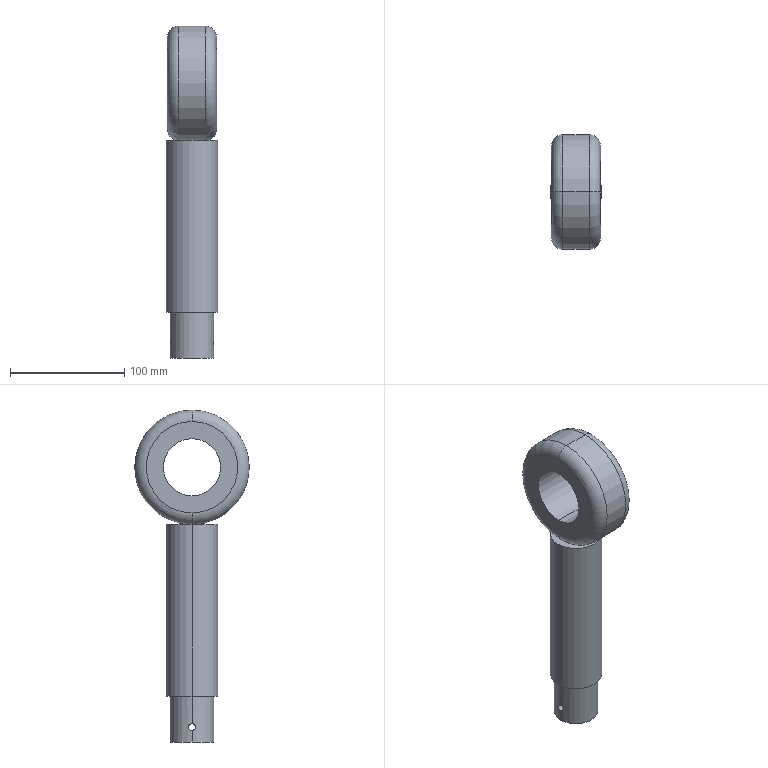Part | SolidWorks | features ICE 3, Extrusion 1, Fillet 1 | 2 solids | 19 faces | box 45 x 100 x 290 mm | volume 523268 mm3 | cylinder 10 | plane 5 | torus 4 | commonest cylinder face diameters 6 x2 38 x2 45 x2 50 x2 100 x2
STEP:
#1=CARTESIAN_POINT('',(11.5,0.,290.));
#2=VERTEX_POINT('',#1);
#3=CARTESIAN_POINT('',(11.5,0.,190.));
#4=VERTEX_POINT('',#3);
#5=CARTESIAN_POINT('',(11.5,0.,240.));
#6=DIRECTION('',(-1.,0.,0.));
#7=DIRECTION('',(0.,0.,-1.));
#8=AXIS2_PLACEMENT_3D('',#5,#6,#7);
#9=CIRCLE('',#8,50.);
#10=EDGE_CURVE('',#2,#4,#9,.T.);
#11=ORIENTED_EDGE('',*,*,#10,.F.);
#12=CARTESIAN_POINT('',(21.5,0.,280.));
#13=VERTEX_POINT('',#12);
#14=CARTESIAN_POINT('',(11.5,0.,280.));
#15=DIRECTION('',(0.,1.,0.));
#16=DIRECTION('',(0.,0.,1.));
#17=AXIS2_PLACEMENT_3D('',#14,#15,#16);
#18=CIRCLE('',#17,10.);
#19=EDGE_CURVE('',#2,#13,#18,.T.);
#20=ORIENTED_EDGE('',*,*,#19,.T.);
#21=CARTESIAN_POINT('',(21.5,0.,200.));
#22=VERTEX_POINT('',#21);
#23=CARTESIAN_POINT('',(21.5,0.,240.));
#24=DIRECTION('',(1.,0.,0.));
#25=DIRECTION('',(0.,0.,-1.));
#26=AXIS2_PLACEMENT_3D('',#23,#24,#25);
#27=CIRCLE('',#26,40.);
#28=EDGE_CURVE('',#22,#13,#27,.T.);
#29=ORIENTED_EDGE('',*,*,#28,.F.);
#30=CARTESIAN_POINT('',(11.5,0.,200.));
#31=DIRECTION('',(0.,-1.,0.));
#32=DIRECTION('',(0.,0.,-1.));
#33=AXIS2_PLACEMENT_3D('',#30,#31,#32);
#34=CIRCLE('',#33,10.);
#35=EDGE_CURVE('',#4,#22,#34,.T.);
#36=ORIENTED_EDGE('',*,*,#35,.F.);
#37=EDGE_LOOP('',(#11,#20,#29,#36));
#38=FACE_OUTER_BOUND('',#37,.T.);
#39=CARTESIAN_POINT('',(11.5,0.,240.));
#40=DIRECTION('',(1.,0.,0.));
#41=DIRECTION('',(0.,0.,-1.));
#42=AXIS2_PLACEMENT_3D('',#39,#40,#41);
#43=TOROIDAL_SURFACE('',#42,40.,10.);
#44=ADVANCED_FACE('',(#38),#43,.T.);
#45=CARTESIAN_POINT('',(-21.5,0.,280.));
#46=VERTEX_POINT('',#45);
#47=CARTESIAN_POINT('',(-21.5,0.,200.));
#48=VERTEX_POINT('',#47);
#49=CARTESIAN_POINT('',(-21.5,0.,240.));
#50=DIRECTION('',(-1.,0.,0.));
#51=DIRECTION('',(0.,0.,-1.));
#52=AXIS2_PLACEMENT_3D('',#49,#50,#51);
#53=CIRCLE('',#52,40.);
#54=EDGE_CURVE('',#46,#48,#53,.T.);
#55=ORIENTED_EDGE('',*,*,#54,.F.);
#56=CARTESIAN_POINT('',(-11.5,0.,290.));
#57=VERTEX_POINT('',#56);
#58=CARTESIAN_POINT('',(-11.5,0.,280.));
#59=DIRECTION('',(0.,1.,0.));
#60=DIRECTION('',(0.,0.,1.));
#61=AXIS2_PLACEMENT_3D('',#58,#59,#60);
#62=CIRCLE('',#61,10.);
#63=EDGE_CURVE('',#46,#57,#62,.T.);
#64=ORIENTED_EDGE('',*,*,#63,.T.);
#65=CARTESIAN_POINT('',(-11.5,0.,190.));
#66=VERTEX_POINT('',#65);
#67=CARTESIAN_POINT('',(-11.5,0.,240.));
#68=DIRECTION('',(1.,0.,0.));
#69=DIRECTION('',(0.,0.,-1.));
#70=AXIS2_PLACEMENT_3D('',#67,#68,#69);
#71=CIRCLE('',#70,50.);
#72=EDGE_CURVE('',#66,#57,#71,.T.);
#73=ORIENTED_EDGE('',*,*,#72,.F.);
#74=CARTESIAN_POINT('',(-11.5,0.,200.));
#75=DIRECTION('',(0.,-1.,0.));
#76=DIRECTION('',(0.,0.,-1.));
#77=AXIS2_PLACEMENT_3D('',#74,#75,#76);
#78=CIRCLE('',#77,10.);
#79=EDGE_CURVE('',#48,#66,#78,.T.);
#80=ORIENTED_EDGE('',*,*,#79,.F.);
#81=EDGE_LOOP('',(#55,#64,#73,#80));
#82=FACE_OUTER_BOUND('',#81,.T.);
#83=CARTESIAN_POINT('',(-11.5,0.,240.));
#84=DIRECTION('',(1.,0.,0.));
#85=DIRECTION('',(0.,0.,-1.));
#86=AXIS2_PLACEMENT_3D('',#83,#84,#85);
#87=TOROIDAL_SURFACE('',#86,40.,10.);
#88=ADVANCED_FACE('',(#82),#87,.T.);
#89=CARTESIAN_POINT('',(21.5,0.,265.));
#90=VERTEX_POINT('',#89);
#91=CARTESIAN_POINT('',(21.5,0.,215.));
#92=VERTEX_POINT('',#91);
#93=CARTESIAN_POINT('',(21.5,0.,240.));
#94=DIRECTION('',(1.,0.,0.));
#95=DIRECTION('',(0.,0.,-1.));
#96=AXIS2_PLACEMENT_3D('',#93,#94,#95);
#97=CIRCLE('',#96,25.);
#98=EDGE_CURVE('',#90,#92,#97,.T.);
#99=ORIENTED_EDGE('',*,*,#98,.T.);
#100=CARTESIAN_POINT('',(-21.5,0.,215.));
#101=VERTEX_POINT('',#100);
#102=CARTESIAN_POINT('',(21.5,0.,215.));
#103=DIRECTION('',(-1.,0.,0.));
#104=VECTOR('',#103,1000.);
#105=LINE('',#102,#104);
#106=EDGE_CURVE('',#92,#101,#105,.T.);
#107=ORIENTED_EDGE('',*,*,#106,.T.);
#108=CARTESIAN_POINT('',(-21.5,0.,265.));
#109=VERTEX_POINT('',#108);
#110=CARTESIAN_POINT('',(-21.5,0.,240.));
#111=DIRECTION('',(1.,0.,0.));
#112=DIRECTION('',(0.,0.,-1.));
#113=AXIS2_PLACEMENT_3D('',#110,#111,#112);
#114=CIRCLE('',#113,25.);
#115=EDGE_CURVE('',#109,#101,#114,.T.);
#116=ORIENTED_EDGE('',*,*,#115,.F.);
#117=CARTESIAN_POINT('',(21.5,0.,265.));
#118=DIRECTION('',(-1.,0.,0.));
#119=VECTOR('',#118,1000.);
#120=LINE('',#117,#119);
#121=EDGE_CURVE('',#90,#109,#120,.T.);
#122=ORIENTED_EDGE('',*,*,#121,.F.);
#123=EDGE_LOOP('',(#99,#107,#116,#122));
#124=FACE_OUTER_BOUND('',#123,.T.);
#125=CARTESIAN_POINT('',(21.5,0.,240.));
#126=DIRECTION('',(-1.,0.,0.));
#127=DIRECTION('',(0.,0.,1.));
#128=AXIS2_PLACEMENT_3D('',#125,#126,#127);
#129=CYLINDRICAL_SURFACE('',#128,25.);
#130=ADVANCED_FACE('',(#124),#129,.F.);
#131=ORIENTED_EDGE('',*,*,#10,.T.);
#132=CARTESIAN_POINT('',(21.5,0.,190.));
#133=DIRECTION('',(-1.,0.,0.));
#134=VECTOR('',#133,1000.);
#135=LINE('',#132,#134);
#136=EDGE_CURVE('',#4,#66,#135,.T.);
#137=ORIENTED_EDGE('',*,*,#136,.T.);
#138=ORIENTED_EDGE('',*,*,#72,.T.);
#139=CARTESIAN_POINT('',(21.5,0.,290.));
#140=DIRECTION('',(-1.,0.,0.));
#141=VECTOR('',#140,1000.);
#142=LINE('',#139,#141);
#143=EDGE_CURVE('',#2,#57,#142,.T.);
#144=ORIENTED_EDGE('',*,*,#143,.F.);
#145=EDGE_LOOP('',(#131,#137,#138,#144));
#146=FACE_OUTER_BOUND('',#145,.T.);
#147=CARTESIAN_POINT('',(21.5,0.,240.));
#148=DIRECTION('',(-1.,0.,0.));
#149=DIRECTION('',(0.,0.,1.));
#150=AXIS2_PLACEMENT_3D('',#147,#148,#149);
#151=CYLINDRICAL_SURFACE('',#150,50.);
#152=ADVANCED_FACE('',(#146),#151,.T.);
#153=ORIENTED_EDGE('',*,*,#28,.T.);
#154=CARTESIAN_POINT('',(21.5,0.,240.));
#155=DIRECTION('',(1.,0.,0.));
#156=DIRECTION('',(0.,0.,-1.));
#157=AXIS2_PLACEMENT_3D('',#154,#155,#156);
#158=CIRCLE('',#157,40.);
#159=EDGE_CURVE('',#13,#22,#158,.T.);
#160=ORIENTED_EDGE('',*,*,#159,.T.);
#161=EDGE_LOOP('',(#153,#160));
#162=FACE_OUTER_BOUND('',#161,.T.);
#163=ORIENTED_EDGE('',*,*,#98,.F.);
#164=CARTESIAN_POINT('',(21.5,0.,240.));
#165=DIRECTION('',(1.,0.,0.));
#166=DIRECTION('',(0.,0.,-1.));
#167=AXIS2_PLACEMENT_3D('',#164,#165,#166);
#168=CIRCLE('',#167,25.);
#169=EDGE_CURVE('',#92,#90,#168,.T.);
#170=ORIENTED_EDGE('',*,*,#169,.F.);
#171=EDGE_LOOP('',(#163,#170));
#172=FACE_BOUND('',#171,.T.);
#173=CARTESIAN_POINT('',(21.5,0.,240.));
#174=DIRECTION('',(1.,0.,0.));
#175=DIRECTION('',(0.,0.,-1.));
#176=AXIS2_PLACEMENT_3D('',#173,#174,#175);
#177=PLANE('',#176);
#178=ADVANCED_FACE('',(#162,#172),#177,.T.);
#179=CARTESIAN_POINT('',(-21.5,0.,240.));
#180=DIRECTION('',(-1.,0.,0.));
#181=DIRECTION('',(0.,0.,-1.));
#182=AXIS2_PLACEMENT_3D('',#179,#180,#181);
#183=CIRCLE('',#182,40.);
#184=EDGE_CURVE('',#48,#46,#183,.T.);
#185=ORIENTED_EDGE('',*,*,#184,.T.);
#186=ORIENTED_EDGE('',*,*,#54,.T.);
#187=EDGE_LOOP('',(#185,#186));
#188=FACE_OUTER_BOUND('',#187,.T.);
#189=ORIENTED_EDGE('',*,*,#115,.T.);
#190=CARTESIAN_POINT('',(-21.5,0.,240.));
#191=DIRECTION('',(1.,0.,0.));
#192=DIRECTION('',(0.,0.,-1.));
#193=AXIS2_PLACEMENT_3D('',#190,#191,#192);
#194=CIRCLE('',#193,25.);
#195=EDGE_CURVE('',#101,#109,#194,.T.);
#196=ORIENTED_EDGE('',*,*,#195,.T.);
#197=EDGE_LOOP('',(#189,#196));
#198=FACE_BOUND('',#197,.T.);
#199=CARTESIAN_POINT('',(-21.5,0.,240.));
#200=DIRECTION('',(1.,0.,0.));
#201=DIRECTION('',(0.,0.,-1.));
#202=AXIS2_PLACEMENT_3D('',#199,#200,#201);
#203=PLANE('',#202);
#204=ADVANCED_FACE('',(#188,#198),#203,.F.);
#205=ORIENTED_EDGE('',*,*,#136,.F.);
#206=CARTESIAN_POINT('',(11.5,0.,240.));
#207=DIRECTION('',(-1.,0.,0.));
#208=DIRECTION('',(0.,0.,-1.));
#209=AXIS2_PLACEMENT_3D('',#206,#207,#208);
#210=CIRCLE('',#209,50.);
#211=EDGE_CURVE('',#4,#2,#210,.T.);
#212=ORIENTED_EDGE('',*,*,#211,.T.);
#213=ORIENTED_EDGE('',*,*,#143,.T.);
#214=CARTESIAN_POINT('',(-11.5,0.,240.));
#215=DIRECTION('',(1.,0.,0.));
#216=DIRECTION('',(0.,0.,-1.));
#217=AXIS2_PLACEMENT_3D('',#214,#215,#216);
#218=CIRCLE('',#217,50.);
#219=EDGE_CURVE('',#57,#66,#218,.T.);
#220=ORIENTED_EDGE('',*,*,#219,.T.);
#221=EDGE_LOOP('',(#205,#212,#213,#220));
#222=FACE_OUTER_BOUND('',#221,.T.);
#223=CARTESIAN_POINT('',(21.5,0.,240.));
#224=DIRECTION('',(-1.,0.,0.));
#225=DIRECTION('',(0.,0.,1.));
#226=AXIS2_PLACEMENT_3D('',#223,#224,#225);
#227=CYLINDRICAL_SURFACE('',#226,50.);
#228=ADVANCED_FACE('',(#222),#227,.T.);
#229=ORIENTED_EDGE('',*,*,#106,.F.);
#230=ORIENTED_EDGE('',*,*,#169,.T.);
#231=ORIENTED_EDGE('',*,*,#121,.T.);
#232=ORIENTED_EDGE('',*,*,#195,.F.);
#233=EDGE_LOOP('',(#229,#230,#231,#232));
#234=FACE_OUTER_BOUND('',#233,.T.);
#235=CARTESIAN_POINT('',(21.5,0.,240.));
#236=DIRECTION('',(-1.,0.,0.));
#237=DIRECTION('',(0.,0.,1.));
#238=AXIS2_PLACEMENT_3D('',#235,#236,#237);
#239=CYLINDRICAL_SURFACE('',#238,25.);
#240=ADVANCED_FACE('',(#234),#239,.F.);
#241=ORIENTED_EDGE('',*,*,#63,.F.);
#242=ORIENTED_EDGE('',*,*,#184,.F.);
#243=ORIENTED_EDGE('',*,*,#79,.T.);
#244=ORIENTED_EDGE('',*,*,#219,.F.);
#245=EDGE_LOOP('',(#241,#242,#243,#244));
#246=FACE_OUTER_BOUND('',#245,.T.);
#247=CARTESIAN_POINT('',(-11.5,0.,240.));
#248=DIRECTION('',(1.,0.,0.));
#249=DIRECTION('',(0.,0.,-1.));
#250=AXIS2_PLACEMENT_3D('',#247,#248,#249);
#251=TOROIDAL_SURFACE('',#250,40.,10.);
#252=ADVANCED_FACE('',(#246),#251,.T.);
#253=ORIENTED_EDGE('',*,*,#19,.F.);
#254=ORIENTED_EDGE('',*,*,#211,.F.);
#255=ORIENTED_EDGE('',*,*,#35,.T.);
#256=ORIENTED_EDGE('',*,*,#159,.F.);
#257=EDGE_LOOP('',(#253,#254,#255,#256));
#258=FACE_OUTER_BOUND('',#257,.T.);
#259=CARTESIAN_POINT('',(11.5,0.,240.));
#260=DIRECTION('',(1.,0.,0.));
#261=DIRECTION('',(0.,0.,-1.));
#262=AXIS2_PLACEMENT_3D('',#259,#260,#261);
#263=TOROIDAL_SURFACE('',#262,40.,10.);
#264=ADVANCED_FACE('',(#258),#263,.T.);
#265=CLOSED_SHELL('',(#44,#88,#130,#152,#178,#204,#228,#240,#252,#264));
#266=MANIFOLD_SOLID_BREP('',#265);
#267=CARTESIAN_POINT('',(-19.,0.,10.));
#268=VERTEX_POINT('',#267);
#269=CARTESIAN_POINT('',(-19.,0.,16.));
#270=VERTEX_POINT('',#269);
#271=CARTESIAN_POINT('',(-19.,0.,10.));
#272=CARTESIAN_POINT('',(-19.,-0.1959,10.));
#273=CARTESIAN_POINT('',(-18.997,-0.3908,10.019));
#274=CARTESIAN_POINT('',(-18.985,-0.7787,10.096));
#275=CARTESIAN_POINT('',(-18.976,-0.9676,10.154));
#276=CARTESIAN_POINT('',(-18.954,-1.329,10.303));
#277=CARTESIAN_POINT('',(-18.941,-1.504,10.397));
#278=CARTESIAN_POINT('',(-18.912,-1.831,10.615));
#279=CARTESIAN_POINT('',(-18.897,-1.982,10.739));
#280=CARTESIAN_POINT('',(-18.866,-2.258,11.015));
#281=CARTESIAN_POINT('',(-18.85,-2.385,11.17));
#282=CARTESIAN_POINT('',(-18.821,-2.602,11.495));
#283=CARTESIAN_POINT('',(-18.808,-2.695,11.667));
#284=CARTESIAN_POINT('',(-18.786,-2.846,12.03));
#285=CARTESIAN_POINT('',(-18.777,-2.904,12.221));
#286=CARTESIAN_POINT('',(-18.765,-2.98,12.604));
#287=CARTESIAN_POINT('',(-18.762,-3.,12.8));
#288=CARTESIAN_POINT('',(-18.762,-3.,13.196));
#289=CARTESIAN_POINT('',(-18.765,-2.981,13.391));
#290=CARTESIAN_POINT('',(-18.777,-2.905,13.775));
#291=CARTESIAN_POINT('',(-18.786,-2.847,13.966));
#292=CARTESIAN_POINT('',(-18.808,-2.697,14.329));
#293=CARTESIAN_POINT('',(-18.821,-2.605,14.501));
#294=CARTESIAN_POINT('',(-18.85,-2.387,14.828));
#295=CARTESIAN_POINT('',(-18.866,-2.261,14.982));
#296=CARTESIAN_POINT('',(-18.897,-1.985,15.258));
#297=CARTESIAN_POINT('',(-18.912,-1.834,15.382));
#298=CARTESIAN_POINT('',(-18.941,-1.506,15.602));
#299=CARTESIAN_POINT('',(-18.954,-1.332,15.695));
#300=CARTESIAN_POINT('',(-18.976,-0.9717,15.845));
#301=CARTESIAN_POINT('',(-18.985,-0.7822,15.903));
#302=CARTESIAN_POINT('',(-18.997,-0.3946,15.98));
#303=CARTESIAN_POINT('',(-19.,-0.1985,16.));
#304=CARTESIAN_POINT('',(-19.,0.,16.));
#305=B_SPLINE_CURVE_WITH_KNOTS('',3,(#271,#272,#273,#274,#275,#276,#277,#278,#279,#280,#281,#282,#283,#284,#285,#286,#287,#288,#289,#290,#291,#292,#293,#294,#295,#296,#297,#298,#299,#300,#301,#302,#303,#304),.UNSPECIFIED.,.F.,.F.,(4,2,2,2,2,2,2,2,2,2,2,2,2,2,2,2,4),(0.009394,0.009981,0.01057,0.01116,0.01174,0.01233,0.01292,0.0135,0.01409,0.01468,0.01526,0.01585,0.01644,0.01702,0.01761,0.0182,0.01879),.UNSPECIFIED.);
#306=EDGE_CURVE('',#268,#270,#305,.T.);
#307=ORIENTED_EDGE('',*,*,#306,.T.);
#308=CARTESIAN_POINT('',(19.,0.,16.));
#309=VERTEX_POINT('',#308);
#310=CARTESIAN_POINT('',(-25.,0.,16.));
#311=DIRECTION('',(1.,0.,0.));
#312=VECTOR('',#311,1000.);
#313=LINE('',#310,#312);
#314=EDGE_CURVE('',#270,#309,#313,.T.);
#315=ORIENTED_EDGE('',*,*,#314,.T.);
#316=CARTESIAN_POINT('',(19.,0.,10.));
#317=VERTEX_POINT('',#316);
#318=CARTESIAN_POINT('',(19.,0.,16.));
#319=CARTESIAN_POINT('',(19.,-0.1959,16.));
#320=CARTESIAN_POINT('',(18.997,-0.3908,15.981));
#321=CARTESIAN_POINT('',(18.985,-0.7787,15.904));
#322=CARTESIAN_POINT('',(18.976,-0.9676,15.846));
#323=CARTESIAN_POINT('',(18.954,-1.329,15.697));
#324=CARTESIAN_POINT('',(18.941,-1.504,15.603));
#325=CARTESIAN_POINT('',(18.912,-1.831,15.385));
#326=CARTESIAN_POINT('',(18.897,-1.982,15.261));
#327=CARTESIAN_POINT('',(18.866,-2.258,14.985));
#328=CARTESIAN_POINT('',(18.85,-2.385,14.83));
#329=CARTESIAN_POINT('',(18.821,-2.602,14.505));
#330=CARTESIAN_POINT('',(18.808,-2.695,14.333));
#331=CARTESIAN_POINT('',(18.786,-2.846,13.97));
#332=CARTESIAN_POINT('',(18.777,-2.904,13.779));
#333=CARTESIAN_POINT('',(18.765,-2.98,13.396));
#334=CARTESIAN_POINT('',(18.762,-3.,13.2));
#335=CARTESIAN_POINT('',(18.762,-3.,12.804));
#336=CARTESIAN_POINT('',(18.765,-2.981,12.609));
#337=CARTESIAN_POINT('',(18.777,-2.905,12.225));
#338=CARTESIAN_POINT('',(18.786,-2.847,12.034));
#339=CARTESIAN_POINT('',(18.808,-2.697,11.671));
#340=CARTESIAN_POINT('',(18.821,-2.605,11.499));
#341=CARTESIAN_POINT('',(18.85,-2.387,11.172));
#342=CARTESIAN_POINT('',(18.866,-2.261,11.018));
#343=CARTESIAN_POINT('',(18.897,-1.985,10.742));
#344=CARTESIAN_POINT('',(18.912,-1.834,10.618));
#345=CARTESIAN_POINT('',(18.941,-1.506,10.398));
#346=CARTESIAN_POINT('',(18.954,-1.332,10.305));
#347=CARTESIAN_POINT('',(18.976,-0.9717,10.155));
#348=CARTESIAN_POINT('',(18.985,-0.7822,10.097));
#349=CARTESIAN_POINT('',(18.997,-0.3946,10.02));
#350=CARTESIAN_POINT('',(19.,-0.1985,10.));
#351=CARTESIAN_POINT('',(19.,0.,10.));
#352=B_SPLINE_CURVE_WITH_KNOTS('',3,(#318,#319,#320,#321,#322,#323,#324,#325,#326,#327,#328,#329,#330,#331,#332,#333,#334,#335,#336,#337,#338,#339,#340,#341,#342,#343,#344,#345,#346,#347,#348,#349,#350,#351),.UNSPECIFIED.,.F.,.F.,(4,2,2,2,2,2,2,2,2,2,2,2,2,2,2,2,4),(0.009394,0.009981,0.01057,0.01116,0.01174,0.01233,0.01292,0.0135,0.01409,0.01468,0.01526,0.01585,0.01644,0.01702,0.01761,0.0182,0.01879),.UNSPECIFIED.);
#353=EDGE_CURVE('',#309,#317,#352,.T.);
#354=ORIENTED_EDGE('',*,*,#353,.T.);
#355=CARTESIAN_POINT('',(-25.,0.,10.));
#356=DIRECTION('',(1.,0.,0.));
#357=VECTOR('',#356,1000.);
#358=LINE('',#355,#357);
#359=EDGE_CURVE('',#268,#317,#358,.T.);
#360=ORIENTED_EDGE('',*,*,#359,.F.);
#361=EDGE_LOOP('',(#307,#315,#354,#360));
#362=FACE_OUTER_BOUND('',#361,.T.);
#363=CARTESIAN_POINT('',(-25.,0.,13.));
#364=DIRECTION('',(1.,0.,0.));
#365=DIRECTION('',(0.,0.,-1.));
#366=AXIS2_PLACEMENT_3D('',#363,#364,#365);
#367=CYLINDRICAL_SURFACE('',#366,3.);
#368=ADVANCED_FACE('',(#362),#367,.F.);
#369=CARTESIAN_POINT('',(-19.,0.,40.));
#370=VERTEX_POINT('',#369);
#371=CARTESIAN_POINT('',(19.,0.,40.));
#372=VERTEX_POINT('',#371);
#373=CARTESIAN_POINT('',(0.,0.,40.));
#374=DIRECTION('',(0.,0.,-1.));
#375=DIRECTION('',(-1.,0.,0.));
#376=AXIS2_PLACEMENT_3D('',#373,#374,#375);
#377=CIRCLE('',#376,19.);
#378=EDGE_CURVE('',#370,#372,#377,.T.);
#379=ORIENTED_EDGE('',*,*,#378,.T.);
#380=CARTESIAN_POINT('',(19.,0.,40.));
#381=DIRECTION('',(0.,0.,-1.));
#382=VECTOR('',#381,1000.);
#383=LINE('',#380,#382);
#384=EDGE_CURVE('',#372,#309,#383,.T.);
#385=ORIENTED_EDGE('',*,*,#384,.T.);
#386=CARTESIAN_POINT('',(19.,0.,10.));
#387=CARTESIAN_POINT('',(19.,0.1986,10.));
#388=CARTESIAN_POINT('',(18.997,0.3937,10.02));
#389=CARTESIAN_POINT('',(18.985,0.7776,10.096));
#390=CARTESIAN_POINT('',(18.976,0.9683,10.154));
#391=CARTESIAN_POINT('',(18.954,1.332,10.304));
#392=CARTESIAN_POINT('',(18.941,1.504,10.397));
#393=CARTESIAN_POINT('',(18.912,1.83,10.614));
#394=CARTESIAN_POINT('',(18.897,1.984,10.741));
#395=CARTESIAN_POINT('',(18.866,2.26,11.017));
#396=CARTESIAN_POINT('',(18.85,2.384,11.168));
#397=CARTESIAN_POINT('',(18.821,2.603,11.496));
#398=CARTESIAN_POINT('',(18.808,2.696,11.67));
#399=CARTESIAN_POINT('',(18.786,2.846,12.031));
#400=CARTESIAN_POINT('',(18.777,2.904,12.221));
#401=CARTESIAN_POINT('',(18.765,2.981,12.608));
#402=CARTESIAN_POINT('',(18.762,3.,12.803));
#403=CARTESIAN_POINT('',(18.762,3.,13.195));
#404=CARTESIAN_POINT('',(18.765,2.98,13.394));
#405=CARTESIAN_POINT('',(18.777,2.904,13.779));
#406=CARTESIAN_POINT('',(18.786,2.847,13.966));
#407=CARTESIAN_POINT('',(18.808,2.696,14.33));
#408=CARTESIAN_POINT('',(18.821,2.603,14.505));
#409=CARTESIAN_POINT('',(18.85,2.385,14.83));
#410=CARTESIAN_POINT('',(18.866,2.261,14.982));
#411=CARTESIAN_POINT('',(18.897,1.982,15.261));
#412=CARTESIAN_POINT('',(18.912,1.83,15.385));
#413=CARTESIAN_POINT('',(18.941,1.506,15.602));
#414=CARTESIAN_POINT('',(18.954,1.33,15.696));
#415=CARTESIAN_POINT('',(18.976,0.9672,15.847));
#416=CARTESIAN_POINT('',(18.985,0.7801,15.903));
#417=CARTESIAN_POINT('',(18.997,0.395,15.98));
#418=CARTESIAN_POINT('',(19.,0.196,16.));
#419=CARTESIAN_POINT('',(19.,0.,16.));
#420=B_SPLINE_CURVE_WITH_KNOTS('',3,(#386,#387,#388,#389,#390,#391,#392,#393,#394,#395,#396,#397,#398,#399,#400,#401,#402,#403,#404,#405,#406,#407,#408,#409,#410,#411,#412,#413,#414,#415,#416,#417,#418,#419),.UNSPECIFIED.,.F.,.F.,(4,2,2,2,2,2,2,2,2,2,2,2,2,2,2,2,4),(0.,0.0005871,0.001174,0.001761,0.002349,0.002936,0.003523,0.00411,0.004697,0.005284,0.005871,0.006458,0.007046,0.007633,0.00822,0.008807,0.009394),.UNSPECIFIED.);
#421=EDGE_CURVE('',#317,#309,#420,.T.);
#422=ORIENTED_EDGE('',*,*,#421,.F.);
#423=CARTESIAN_POINT('',(19.,0.,0.));
#424=VERTEX_POINT('',#423);
#425=CARTESIAN_POINT('',(19.,0.,40.));
#426=DIRECTION('',(0.,0.,-1.));
#427=VECTOR('',#426,1000.);
#428=LINE('',#425,#427);
#429=EDGE_CURVE('',#317,#424,#428,.T.);
#430=ORIENTED_EDGE('',*,*,#429,.T.);
#431=CARTESIAN_POINT('',(-19.,0.,0.));
#432=VERTEX_POINT('',#431);
#433=CARTESIAN_POINT('',(0.,0.,0.));
#434=DIRECTION('',(0.,0.,-1.));
#435=DIRECTION('',(-1.,0.,0.));
#436=AXIS2_PLACEMENT_3D('',#433,#434,#435);
#437=CIRCLE('',#436,19.);
#438=EDGE_CURVE('',#432,#424,#437,.T.);
#439=ORIENTED_EDGE('',*,*,#438,.F.);
#440=CARTESIAN_POINT('',(-19.,0.,40.));
#441=DIRECTION('',(0.,0.,-1.));
#442=VECTOR('',#441,1000.);
#443=LINE('',#440,#442);
#444=EDGE_CURVE('',#268,#432,#443,.T.);
#445=ORIENTED_EDGE('',*,*,#444,.F.);
#446=CARTESIAN_POINT('',(-19.,0.,16.));
#447=CARTESIAN_POINT('',(-19.,0.1986,16.));
#448=CARTESIAN_POINT('',(-18.997,0.3937,15.98));
#449=CARTESIAN_POINT('',(-18.985,0.7776,15.904));
#450=CARTESIAN_POINT('',(-18.976,0.9683,15.846));
#451=CARTESIAN_POINT('',(-18.954,1.332,15.696));
#452=CARTESIAN_POINT('',(-18.941,1.504,15.603));
#453=CARTESIAN_POINT('',(-18.912,1.83,15.386));
#454=CARTESIAN_POINT('',(-18.897,1.984,15.259));
#455=CARTESIAN_POINT('',(-18.866,2.26,14.983));
#456=CARTESIAN_POINT('',(-18.85,2.384,14.832));
#457=CARTESIAN_POINT('',(-18.821,2.603,14.504));
#458=CARTESIAN_POINT('',(-18.808,2.696,14.33));
#459=CARTESIAN_POINT('',(-18.786,2.846,13.969));
#460=CARTESIAN_POINT('',(-18.777,2.904,13.779));
#461=CARTESIAN_POINT('',(-18.765,2.981,13.392));
#462=CARTESIAN_POINT('',(-18.762,3.,13.197));
#463=CARTESIAN_POINT('',(-18.762,3.,12.805));
#464=CARTESIAN_POINT('',(-18.765,2.98,12.606));
#465=CARTESIAN_POINT('',(-18.777,2.904,12.221));
#466=CARTESIAN_POINT('',(-18.786,2.847,12.034));
#467=CARTESIAN_POINT('',(-18.808,2.696,11.67));
#468=CARTESIAN_POINT('',(-18.821,2.603,11.495));
#469=CARTESIAN_POINT('',(-18.85,2.385,11.17));
#470=CARTESIAN_POINT('',(-18.866,2.261,11.018));
#471=CARTESIAN_POINT('',(-18.897,1.982,10.739));
#472=CARTESIAN_POINT('',(-18.912,1.83,10.615));
#473=CARTESIAN_POINT('',(-18.941,1.506,10.398));
#474=CARTESIAN_POINT('',(-18.954,1.33,10.304));
#475=CARTESIAN_POINT('',(-18.976,0.9672,10.153));
#476=CARTESIAN_POINT('',(-18.985,0.7801,10.097));
#477=CARTESIAN_POINT('',(-18.997,0.395,10.02));
#478=CARTESIAN_POINT('',(-19.,0.196,10.));
#479=CARTESIAN_POINT('',(-19.,0.,10.));
#480=B_SPLINE_CURVE_WITH_KNOTS('',3,(#446,#447,#448,#449,#450,#451,#452,#453,#454,#455,#456,#457,#458,#459,#460,#461,#462,#463,#464,#465,#466,#467,#468,#469,#470,#471,#472,#473,#474,#475,#476,#477,#478,#479),.UNSPECIFIED.,.F.,.F.,(4,2,2,2,2,2,2,2,2,2,2,2,2,2,2,2,4),(0.,0.0005871,0.001174,0.001761,0.002349,0.002936,0.003523,0.00411,0.004697,0.005284,0.005871,0.006458,0.007046,0.007633,0.00822,0.008807,0.009394),.UNSPECIFIED.);
#481=EDGE_CURVE('',#270,#268,#480,.T.);
#482=ORIENTED_EDGE('',*,*,#481,.F.);
#483=CARTESIAN_POINT('',(-19.,0.,40.));
#484=DIRECTION('',(0.,0.,-1.));
#485=VECTOR('',#484,1000.);
#486=LINE('',#483,#485);
#487=EDGE_CURVE('',#370,#270,#486,.T.);
#488=ORIENTED_EDGE('',*,*,#487,.F.);
#489=EDGE_LOOP('',(#379,#385,#422,#430,#439,#445,#482,#488));
#490=FACE_OUTER_BOUND('',#489,.T.);
#491=CARTESIAN_POINT('',(0.,0.,40.));
#492=DIRECTION('',(0.,0.,-1.));
#493=DIRECTION('',(-1.,0.,0.));
#494=AXIS2_PLACEMENT_3D('',#491,#492,#493);
#495=CYLINDRICAL_SURFACE('',#494,19.);
#496=ADVANCED_FACE('',(#490),#495,.T.);
#497=CARTESIAN_POINT('',(22.5,0.,190.));
#498=VERTEX_POINT('',#497);
#499=CARTESIAN_POINT('',(-22.5,0.,190.));
#500=VERTEX_POINT('',#499);
#501=CARTESIAN_POINT('',(0.,0.,190.));
#502=DIRECTION('',(0.,0.,1.));
#503=DIRECTION('',(1.,0.,0.));
#504=AXIS2_PLACEMENT_3D('',#501,#502,#503);
#505=CIRCLE('',#504,22.5);
#506=EDGE_CURVE('',#498,#500,#505,.T.);
#507=ORIENTED_EDGE('',*,*,#506,.F.);
#508=CARTESIAN_POINT('',(22.5,0.,40.));
#509=VERTEX_POINT('',#508);
#510=CARTESIAN_POINT('',(22.5,0.,190.));
#511=DIRECTION('',(0.,0.,-1.));
#512=VECTOR('',#511,1000.);
#513=LINE('',#510,#512);
#514=EDGE_CURVE('',#498,#509,#513,.T.);
#515=ORIENTED_EDGE('',*,*,#514,.T.);
#516=CARTESIAN_POINT('',(-22.5,0.,40.));
#517=VERTEX_POINT('',#516);
#518=CARTESIAN_POINT('',(0.,0.,40.));
#519=DIRECTION('',(0.,0.,-1.));
#520=DIRECTION('',(-1.,0.,0.));
#521=AXIS2_PLACEMENT_3D('',#518,#519,#520);
#522=CIRCLE('',#521,22.5);
#523=EDGE_CURVE('',#517,#509,#522,.T.);
#524=ORIENTED_EDGE('',*,*,#523,.F.);
#525=CARTESIAN_POINT('',(-22.5,0.,190.));
#526=DIRECTION('',(0.,0.,-1.));
#527=VECTOR('',#526,1000.);
#528=LINE('',#525,#527);
#529=EDGE_CURVE('',#500,#517,#528,.T.);
#530=ORIENTED_EDGE('',*,*,#529,.F.);
#531=EDGE_LOOP('',(#507,#515,#524,#530));
#532=FACE_OUTER_BOUND('',#531,.T.);
#533=CARTESIAN_POINT('',(0.,0.,190.));
#534=DIRECTION('',(0.,0.,-1.));
#535=DIRECTION('',(-1.,0.,0.));
#536=AXIS2_PLACEMENT_3D('',#533,#534,#535);
#537=CYLINDRICAL_SURFACE('',#536,22.5);
#538=ADVANCED_FACE('',(#532),#537,.T.);
#539=ORIENTED_EDGE('',*,*,#514,.F.);
#540=CARTESIAN_POINT('',(0.,0.,190.));
#541=DIRECTION('',(0.,0.,1.));
#542=DIRECTION('',(1.,0.,0.));
#543=AXIS2_PLACEMENT_3D('',#540,#541,#542);
#544=CIRCLE('',#543,22.5);
#545=EDGE_CURVE('',#500,#498,#544,.T.);
#546=ORIENTED_EDGE('',*,*,#545,.F.);
#547=ORIENTED_EDGE('',*,*,#529,.T.);
#548=CARTESIAN_POINT('',(0.,0.,40.));
#549=DIRECTION('',(0.,0.,-1.));
#550=DIRECTION('',(-1.,0.,0.));
#551=AXIS2_PLACEMENT_3D('',#548,#549,#550);
#552=CIRCLE('',#551,22.5);
#553=EDGE_CURVE('',#509,#517,#552,.T.);
#554=ORIENTED_EDGE('',*,*,#553,.F.);
#555=EDGE_LOOP('',(#539,#546,#547,#554));
#556=FACE_OUTER_BOUND('',#555,.T.);
#557=CARTESIAN_POINT('',(0.,0.,190.));
#558=DIRECTION('',(0.,0.,-1.));
#559=DIRECTION('',(-1.,0.,0.));
#560=AXIS2_PLACEMENT_3D('',#557,#558,#559);
#561=CYLINDRICAL_SURFACE('',#560,22.5);
#562=ADVANCED_FACE('',(#556),#561,.T.);
#563=ORIENTED_EDGE('',*,*,#545,.T.);
#564=ORIENTED_EDGE('',*,*,#506,.T.);
#565=EDGE_LOOP('',(#563,#564));
#566=FACE_OUTER_BOUND('',#565,.T.);
#567=CARTESIAN_POINT('',(0.,0.,190.));
#568=DIRECTION('',(0.,0.,1.));
#569=DIRECTION('',(1.,0.,0.));
#570=AXIS2_PLACEMENT_3D('',#567,#568,#569);
#571=PLANE('',#570);
#572=ADVANCED_FACE('',(#566),#571,.T.);
#573=ORIENTED_EDGE('',*,*,#378,.F.);
#574=CARTESIAN_POINT('',(0.,0.,40.));
#575=DIRECTION('',(0.,0.,-1.));
#576=DIRECTION('',(-1.,0.,0.));
#577=AXIS2_PLACEMENT_3D('',#574,#575,#576);
#578=CIRCLE('',#577,19.);
#579=EDGE_CURVE('',#372,#370,#578,.T.);
#580=ORIENTED_EDGE('',*,*,#579,.F.);
#581=EDGE_LOOP('',(#573,#580));
#582=FACE_BOUND('',#581,.T.);
#583=ORIENTED_EDGE('',*,*,#523,.T.);
#584=ORIENTED_EDGE('',*,*,#553,.T.);
#585=EDGE_LOOP('',(#583,#584));
#586=FACE_OUTER_BOUND('',#585,.T.);
#587=CARTESIAN_POINT('',(0.,0.,40.));
#588=DIRECTION('',(0.,0.,-1.));
#589=DIRECTION('',(-1.,0.,0.));
#590=AXIS2_PLACEMENT_3D('',#587,#588,#589);
#591=PLANE('',#590);
#592=ADVANCED_FACE('',(#582,#586),#591,.T.);
#593=ORIENTED_EDGE('',*,*,#384,.F.);
#594=ORIENTED_EDGE('',*,*,#579,.T.);
#595=ORIENTED_EDGE('',*,*,#487,.T.);
#596=ORIENTED_EDGE('',*,*,#306,.F.);
#597=ORIENTED_EDGE('',*,*,#444,.T.);
#598=CARTESIAN_POINT('',(0.,0.,0.));
#599=DIRECTION('',(0.,0.,-1.));
#600=DIRECTION('',(-1.,0.,0.));
#601=AXIS2_PLACEMENT_3D('',#598,#599,#600);
#602=CIRCLE('',#601,19.);
#603=EDGE_CURVE('',#424,#432,#602,.T.);
#604=ORIENTED_EDGE('',*,*,#603,.F.);
#605=ORIENTED_EDGE('',*,*,#429,.F.);
#606=ORIENTED_EDGE('',*,*,#353,.F.);
#607=EDGE_LOOP('',(#593,#594,#595,#596,#597,#604,#605,#606));
#608=FACE_OUTER_BOUND('',#607,.T.);
#609=CARTESIAN_POINT('',(0.,0.,40.));
#610=DIRECTION('',(0.,0.,-1.));
#611=DIRECTION('',(-1.,0.,0.));
#612=AXIS2_PLACEMENT_3D('',#609,#610,#611);
#613=CYLINDRICAL_SURFACE('',#612,19.);
#614=ADVANCED_FACE('',(#608),#613,.T.);
#615=ORIENTED_EDGE('',*,*,#438,.T.);
#616=ORIENTED_EDGE('',*,*,#603,.T.);
#617=EDGE_LOOP('',(#615,#616));
#618=FACE_OUTER_BOUND('',#617,.T.);
#619=CARTESIAN_POINT('',(0.,0.,0.));
#620=DIRECTION('',(0.,0.,1.));
#621=DIRECTION('',(1.,0.,0.));
#622=AXIS2_PLACEMENT_3D('',#619,#620,#621);
#623=PLANE('',#622);
#624=ADVANCED_FACE('',(#618),#623,.F.);
#625=ORIENTED_EDGE('',*,*,#314,.F.);
#626=ORIENTED_EDGE('',*,*,#481,.T.);
#627=ORIENTED_EDGE('',*,*,#359,.T.);
#628=ORIENTED_EDGE('',*,*,#421,.T.);
#629=EDGE_LOOP('',(#625,#626,#627,#628));
#630=FACE_OUTER_BOUND('',#629,.T.);
#631=CARTESIAN_POINT('',(-25.,0.,13.));
#632=DIRECTION('',(1.,0.,0.));
#633=DIRECTION('',(0.,0.,-1.));
#634=AXIS2_PLACEMENT_3D('',#631,#632,#633);
#635=CYLINDRICAL_SURFACE('',#634,3.);
#636=ADVANCED_FACE('',(#630),#635,.F.);
#637=CLOSED_SHELL('',(#368,#496,#538,#562,#572,#592,#614,#624,#636));
#638=MANIFOLD_SOLID_BREP('',#637);
#639=CARTESIAN_POINT('',(0.,0.,0.));
#640=DIRECTION('',(0.,0.,1.));
#641=DIRECTION('',(1.,0.,0.));
#642=AXIS2_PLACEMENT_3D('',#639,#640,#641);
#643=(LENGTH_UNIT()NAMED_UNIT(*)SI_UNIT(.MILLI.,.METRE.));
#644=UNCERTAINTY_MEASURE_WITH_UNIT(LENGTH_MEASURE(0.00001),#643,'','');
#645=(NAMED_UNIT(*)PLANE_ANGLE_UNIT()SI_UNIT($,.RADIAN.));
#646=(NAMED_UNIT(*)SI_UNIT($,.STERADIAN.)SOLID_ANGLE_UNIT());
#647=(GEOMETRIC_REPRESENTATION_CONTEXT(3)GLOBAL_UNCERTAINTY_ASSIGNED_CONTEXT((#644))GLOBAL_UNIT_ASSIGNED_CONTEXT((#643,#645,#646))REPRESENTATION_CONTEXT('',''));
#648=ADVANCED_BREP_SHAPE_REPRESENTATION('',(#266,#638,#642),#647);